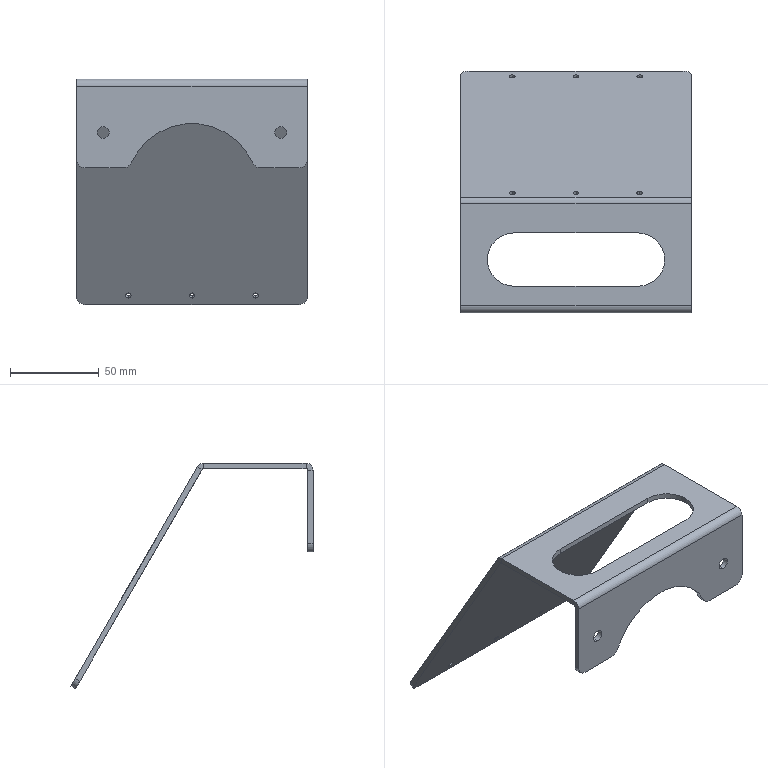Part | STEP file | junction box mounting plate | 1 solid | 51 faces | box 130 x 136.5 x 127.074 mm | volume 85918 mm3 | cylinder 30 | plane 21 | commonest cylinder face diameters 3.3 x12 10 x6 6.6 x4 30 x3 2 x2 8 x2